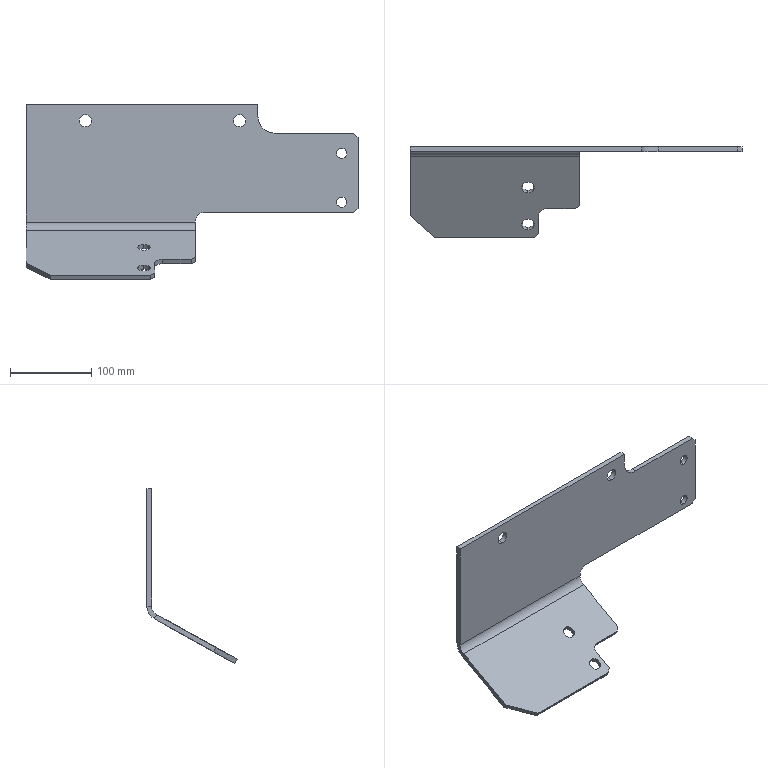Part | SolidWorks | features ICE 2, Chamfer 1, FlatPattern 1, SMBaseFlange 1, SheetMetal 1 | 1 solid | 40 faces | box 408 x 110.914 x 215 mm | volume 454933 mm3 | plane 23 | cylinder 17 | commonest cylinder face diameters 15 x8 12.5 x4 20 x2 24 x1 36 x1 40 x1
STEP:
#1=CARTESIAN_POINT('',(145.,-56.279,-179.402));
#2=VERTEX_POINT('',#1);
#3=CARTESIAN_POINT('',(145.,-43.167,-172.118));
#4=VERTEX_POINT('',#3);
#5=CARTESIAN_POINT('',(145.,-49.723,-175.76));
#6=DIRECTION('',(0.,0.4856,-0.8742));
#7=DIRECTION('',(0.,0.8742,0.4856));
#8=AXIS2_PLACEMENT_3D('',#5,#6,#7);
#9=CIRCLE('',#8,7.5);
#10=EDGE_CURVE('',#2,#4,#9,.T.);
#11=ORIENTED_EDGE('',*,*,#10,.F.);
#12=CARTESIAN_POINT('',(145.,-53.365,-184.647));
#13=VERTEX_POINT('',#12);
#14=CARTESIAN_POINT('',(145.,-145.326,-19.118));
#15=DIRECTION('',(0.,0.4856,-0.8742));
#16=VECTOR('',#15,1000.);
#17=LINE('',#14,#16);
#18=EDGE_CURVE('',#2,#13,#17,.T.);
#19=ORIENTED_EDGE('',*,*,#18,.T.);
#20=CARTESIAN_POINT('',(145.,-40.253,-177.363));
#21=VERTEX_POINT('',#20);
#22=CARTESIAN_POINT('',(145.,-46.809,-181.005));
#23=DIRECTION('',(0.,0.4856,-0.8742));
#24=DIRECTION('',(0.,0.8742,0.4856));
#25=AXIS2_PLACEMENT_3D('',#22,#23,#24);
#26=CIRCLE('',#25,7.5);
#27=EDGE_CURVE('',#13,#21,#26,.T.);
#28=ORIENTED_EDGE('',*,*,#27,.T.);
#29=CARTESIAN_POINT('',(145.,-132.214,-11.833));
#30=DIRECTION('',(0.,0.4856,-0.8742));
#31=VECTOR('',#30,1000.);
#32=LINE('',#29,#31);
#33=EDGE_CURVE('',#4,#21,#32,.T.);
#34=ORIENTED_EDGE('',*,*,#33,.F.);
#35=EDGE_LOOP('',(#11,#19,#28,#34));
#36=FACE_OUTER_BOUND('',#35,.T.);
#37=CARTESIAN_POINT('',(145.,-138.77,-15.476));
#38=DIRECTION('',(0.,0.4856,-0.8742));
#39=DIRECTION('',(0.,0.8742,0.4856));
#40=AXIS2_PLACEMENT_3D('',#37,#38,#39);
#41=CYLINDRICAL_SURFACE('',#40,7.5);
#42=ADVANCED_FACE('',(#36),#41,.F.);
#43=CARTESIAN_POINT('',(145.,-101.735,-204.656));
#44=VERTEX_POINT('',#43);
#45=CARTESIAN_POINT('',(145.,-88.623,-197.371));
#46=VERTEX_POINT('',#45);
#47=CARTESIAN_POINT('',(145.,-95.179,-201.013));
#48=DIRECTION('',(0.,0.4856,-0.8742));
#49=DIRECTION('',(0.,0.8742,0.4856));
#50=AXIS2_PLACEMENT_3D('',#47,#48,#49);
#51=CIRCLE('',#50,7.5);
#52=EDGE_CURVE('',#44,#46,#51,.T.);
#53=ORIENTED_EDGE('',*,*,#52,.F.);
#54=CARTESIAN_POINT('',(145.,-98.821,-209.901));
#55=VERTEX_POINT('',#54);
#56=CARTESIAN_POINT('',(145.,-190.782,-44.371));
#57=DIRECTION('',(0.,0.4856,-0.8742));
#58=VECTOR('',#57,1000.);
#59=LINE('',#56,#58);
#60=EDGE_CURVE('',#44,#55,#59,.T.);
#61=ORIENTED_EDGE('',*,*,#60,.T.);
#62=CARTESIAN_POINT('',(145.,-85.709,-202.616));
#63=VERTEX_POINT('',#62);
#64=CARTESIAN_POINT('',(145.,-92.265,-206.258));
#65=DIRECTION('',(0.,0.4856,-0.8742));
#66=DIRECTION('',(0.,0.8742,0.4856));
#67=AXIS2_PLACEMENT_3D('',#64,#65,#66);
#68=CIRCLE('',#67,7.5);
#69=EDGE_CURVE('',#55,#63,#68,.T.);
#70=ORIENTED_EDGE('',*,*,#69,.T.);
#71=CARTESIAN_POINT('',(145.,-177.67,-37.087));
#72=DIRECTION('',(0.,0.4856,-0.8742));
#73=VECTOR('',#72,1000.);
#74=LINE('',#71,#73);
#75=EDGE_CURVE('',#46,#63,#74,.T.);
#76=ORIENTED_EDGE('',*,*,#75,.F.);
#77=EDGE_LOOP('',(#53,#61,#70,#76));
#78=FACE_OUTER_BOUND('',#77,.T.);
#79=CARTESIAN_POINT('',(145.,-184.226,-40.729));
#80=DIRECTION('',(0.,0.4856,-0.8742));
#81=DIRECTION('',(0.,0.8742,0.4856));
#82=AXIS2_PLACEMENT_3D('',#79,#80,#81);
#83=CYLINDRICAL_SURFACE('',#82,7.5);
#84=ADVANCED_FACE('',(#78),#83,.F.);
#85=CARTESIAN_POINT('',(73.,-6.,-27.5));
#86=VERTEX_POINT('',#85);
#87=CARTESIAN_POINT('',(73.,-6.,-12.5));
#88=VERTEX_POINT('',#87);
#89=CARTESIAN_POINT('',(73.,-6.,-20.));
#90=DIRECTION('',(0.,1.,0.));
#91=DIRECTION('',(0.,0.,1.));
#92=AXIS2_PLACEMENT_3D('',#89,#90,#91);
#93=CIRCLE('',#92,7.5);
#94=EDGE_CURVE('',#86,#88,#93,.T.);
#95=ORIENTED_EDGE('',*,*,#94,.F.);
#96=CARTESIAN_POINT('',(73.,0.,-27.5));
#97=VERTEX_POINT('',#96);
#98=CARTESIAN_POINT('',(73.,-110.914,-27.5));
#99=DIRECTION('',(0.,1.,0.));
#100=VECTOR('',#99,1000.);
#101=LINE('',#98,#100);
#102=EDGE_CURVE('',#86,#97,#101,.T.);
#103=ORIENTED_EDGE('',*,*,#102,.T.);
#104=CARTESIAN_POINT('',(73.,0.,-12.5));
#105=VERTEX_POINT('',#104);
#106=CARTESIAN_POINT('',(73.,0.,-20.));
#107=DIRECTION('',(0.,1.,0.));
#108=DIRECTION('',(0.,0.,1.));
#109=AXIS2_PLACEMENT_3D('',#106,#107,#108);
#110=CIRCLE('',#109,7.5);
#111=EDGE_CURVE('',#97,#105,#110,.T.);
#112=ORIENTED_EDGE('',*,*,#111,.T.);
#113=CARTESIAN_POINT('',(73.,-110.914,-12.5));
#114=DIRECTION('',(0.,1.,0.));
#115=VECTOR('',#114,1000.);
#116=LINE('',#113,#115);
#117=EDGE_CURVE('',#88,#105,#116,.T.);
#118=ORIENTED_EDGE('',*,*,#117,.F.);
#119=EDGE_LOOP('',(#95,#103,#112,#118));
#120=FACE_OUTER_BOUND('',#119,.T.);
#121=CARTESIAN_POINT('',(73.,-110.914,-20.));
#122=DIRECTION('',(0.,1.,0.));
#123=DIRECTION('',(0.,0.,1.));
#124=AXIS2_PLACEMENT_3D('',#121,#122,#123);
#125=CYLINDRICAL_SURFACE('',#124,7.5);
#126=ADVANCED_FACE('',(#120),#125,.F.);
#127=CARTESIAN_POINT('',(388.,-6.,-126.25));
#128=VERTEX_POINT('',#127);
#129=CARTESIAN_POINT('',(388.,-6.,-113.75));
#130=VERTEX_POINT('',#129);
#131=CARTESIAN_POINT('',(388.,-6.,-120.));
#132=DIRECTION('',(0.,1.,0.));
#133=DIRECTION('',(0.,0.,1.));
#134=AXIS2_PLACEMENT_3D('',#131,#132,#133);
#135=CIRCLE('',#134,6.25);
#136=EDGE_CURVE('',#128,#130,#135,.T.);
#137=ORIENTED_EDGE('',*,*,#136,.F.);
#138=CARTESIAN_POINT('',(388.,0.,-126.25));
#139=VERTEX_POINT('',#138);
#140=CARTESIAN_POINT('',(388.,-110.914,-126.25));
#141=DIRECTION('',(0.,1.,0.));
#142=VECTOR('',#141,1000.);
#143=LINE('',#140,#142);
#144=EDGE_CURVE('',#128,#139,#143,.T.);
#145=ORIENTED_EDGE('',*,*,#144,.T.);
#146=CARTESIAN_POINT('',(388.,0.,-113.75));
#147=VERTEX_POINT('',#146);
#148=CARTESIAN_POINT('',(388.,0.,-120.));
#149=DIRECTION('',(0.,1.,0.));
#150=DIRECTION('',(0.,0.,1.));
#151=AXIS2_PLACEMENT_3D('',#148,#149,#150);
#152=CIRCLE('',#151,6.25);
#153=EDGE_CURVE('',#139,#147,#152,.T.);
#154=ORIENTED_EDGE('',*,*,#153,.T.);
#155=CARTESIAN_POINT('',(388.,-110.914,-113.75));
#156=DIRECTION('',(0.,1.,0.));
#157=VECTOR('',#156,1000.);
#158=LINE('',#155,#157);
#159=EDGE_CURVE('',#130,#147,#158,.T.);
#160=ORIENTED_EDGE('',*,*,#159,.F.);
#161=EDGE_LOOP('',(#137,#145,#154,#160));
#162=FACE_OUTER_BOUND('',#161,.T.);
#163=CARTESIAN_POINT('',(388.,-110.914,-120.));
#164=DIRECTION('',(0.,1.,0.));
#165=DIRECTION('',(0.,0.,1.));
#166=AXIS2_PLACEMENT_3D('',#163,#164,#165);
#167=CYLINDRICAL_SURFACE('',#166,6.25);
#168=ADVANCED_FACE('',(#162),#167,.F.);
#169=CARTESIAN_POINT('',(388.,-6.,-66.25));
#170=VERTEX_POINT('',#169);
#171=CARTESIAN_POINT('',(388.,-6.,-53.75));
#172=VERTEX_POINT('',#171);
#173=CARTESIAN_POINT('',(388.,-6.,-60.));
#174=DIRECTION('',(0.,1.,0.));
#175=DIRECTION('',(0.,0.,1.));
#176=AXIS2_PLACEMENT_3D('',#173,#174,#175);
#177=CIRCLE('',#176,6.25);
#178=EDGE_CURVE('',#170,#172,#177,.T.);
#179=ORIENTED_EDGE('',*,*,#178,.F.);
#180=CARTESIAN_POINT('',(388.,0.,-66.25));
#181=VERTEX_POINT('',#180);
#182=CARTESIAN_POINT('',(388.,-110.914,-66.25));
#183=DIRECTION('',(0.,1.,0.));
#184=VECTOR('',#183,1000.);
#185=LINE('',#182,#184);
#186=EDGE_CURVE('',#170,#181,#185,.T.);
#187=ORIENTED_EDGE('',*,*,#186,.T.);
#188=CARTESIAN_POINT('',(388.,0.,-53.75));
#189=VERTEX_POINT('',#188);
#190=CARTESIAN_POINT('',(388.,0.,-60.));
#191=DIRECTION('',(0.,1.,0.));
#192=DIRECTION('',(0.,0.,1.));
#193=AXIS2_PLACEMENT_3D('',#190,#191,#192);
#194=CIRCLE('',#193,6.25);
#195=EDGE_CURVE('',#181,#189,#194,.T.);
#196=ORIENTED_EDGE('',*,*,#195,.T.);
#197=CARTESIAN_POINT('',(388.,-110.914,-53.75));
#198=DIRECTION('',(0.,1.,0.));
#199=VECTOR('',#198,1000.);
#200=LINE('',#197,#199);
#201=EDGE_CURVE('',#172,#189,#200,.T.);
#202=ORIENTED_EDGE('',*,*,#201,.F.);
#203=EDGE_LOOP('',(#179,#187,#196,#202));
#204=FACE_OUTER_BOUND('',#203,.T.);
#205=CARTESIAN_POINT('',(388.,-110.914,-60.));
#206=DIRECTION('',(0.,1.,0.));
#207=DIRECTION('',(0.,0.,1.));
#208=AXIS2_PLACEMENT_3D('',#205,#206,#207);
#209=CYLINDRICAL_SURFACE('',#208,6.25);
#210=ADVANCED_FACE('',(#204),#209,.F.);
#211=CARTESIAN_POINT('',(262.5,-6.,-27.5));
#212=VERTEX_POINT('',#211);
#213=CARTESIAN_POINT('',(262.5,-6.,-12.5));
#214=VERTEX_POINT('',#213);
#215=CARTESIAN_POINT('',(262.5,-6.,-20.));
#216=DIRECTION('',(0.,1.,0.));
#217=DIRECTION('',(0.,0.,1.));
#218=AXIS2_PLACEMENT_3D('',#215,#216,#217);
#219=CIRCLE('',#218,7.5);
#220=EDGE_CURVE('',#212,#214,#219,.T.);
#221=ORIENTED_EDGE('',*,*,#220,.F.);
#222=CARTESIAN_POINT('',(262.5,0.,-27.5));
#223=VERTEX_POINT('',#222);
#224=CARTESIAN_POINT('',(262.5,-110.914,-27.5));
#225=DIRECTION('',(0.,1.,0.));
#226=VECTOR('',#225,1000.);
#227=LINE('',#224,#226);
#228=EDGE_CURVE('',#212,#223,#227,.T.);
#229=ORIENTED_EDGE('',*,*,#228,.T.);
#230=CARTESIAN_POINT('',(262.5,0.,-12.5));
#231=VERTEX_POINT('',#230);
#232=CARTESIAN_POINT('',(262.5,0.,-20.));
#233=DIRECTION('',(0.,1.,0.));
#234=DIRECTION('',(0.,0.,1.));
#235=AXIS2_PLACEMENT_3D('',#232,#233,#234);
#236=CIRCLE('',#235,7.5);
#237=EDGE_CURVE('',#223,#231,#236,.T.);
#238=ORIENTED_EDGE('',*,*,#237,.T.);
#239=CARTESIAN_POINT('',(262.5,-110.914,-12.5));
#240=DIRECTION('',(0.,1.,0.));
#241=VECTOR('',#240,1000.);
#242=LINE('',#239,#241);
#243=EDGE_CURVE('',#214,#231,#242,.T.);
#244=ORIENTED_EDGE('',*,*,#243,.F.);
#245=EDGE_LOOP('',(#221,#229,#238,#244));
#246=FACE_OUTER_BOUND('',#245,.T.);
#247=CARTESIAN_POINT('',(262.5,-110.914,-20.));
#248=DIRECTION('',(0.,1.,0.));
#249=DIRECTION('',(0.,0.,1.));
#250=AXIS2_PLACEMENT_3D('',#247,#248,#249);
#251=CYLINDRICAL_SURFACE('',#250,7.5);
#252=ADVANCED_FACE('',(#246),#251,.F.);
#253=CARTESIAN_POINT('',(208.,-6.,-144.409));
#254=VERTEX_POINT('',#253);
#255=CARTESIAN_POINT('',(208.,-6.,-143.));
#256=VERTEX_POINT('',#255);
#257=CARTESIAN_POINT('',(208.,-6.,0.));
#258=DIRECTION('',(0.,0.,1.));
#259=VECTOR('',#258,1000.);
#260=LINE('',#257,#259);
#261=EDGE_CURVE('',#254,#256,#260,.T.);
#262=ORIENTED_EDGE('',*,*,#261,.F.);
#263=CARTESIAN_POINT('',(208.,0.,-144.409));
#264=VERTEX_POINT('',#263);
#265=CARTESIAN_POINT('',(208.,-6.,-144.409));
#266=DIRECTION('',(0.,1.,0.));
#267=VECTOR('',#266,1000.);
#268=LINE('',#265,#267);
#269=EDGE_CURVE('',#254,#264,#268,.T.);
#270=ORIENTED_EDGE('',*,*,#269,.T.);
#271=CARTESIAN_POINT('',(208.,0.,-143.));
#272=VERTEX_POINT('',#271);
#273=CARTESIAN_POINT('',(208.,0.,-143.));
#274=DIRECTION('',(0.,0.,1.));
#275=VECTOR('',#274,1000.);
#276=LINE('',#273,#275);
#277=EDGE_CURVE('',#264,#272,#276,.T.);
#278=ORIENTED_EDGE('',*,*,#277,.T.);
#279=CARTESIAN_POINT('',(208.,-110.914,-143.));
#280=DIRECTION('',(0.,1.,0.));
#281=VECTOR('',#280,1000.);
#282=LINE('',#279,#281);
#283=EDGE_CURVE('',#256,#272,#282,.T.);
#284=ORIENTED_EDGE('',*,*,#283,.F.);
#285=EDGE_LOOP('',(#262,#270,#278,#284));
#286=FACE_OUTER_BOUND('',#285,.T.);
#287=CARTESIAN_POINT('',(208.,-110.914,-143.));
#288=DIRECTION('',(-1.,0.,0.));
#289=DIRECTION('',(0.,0.,1.));
#290=AXIS2_PLACEMENT_3D('',#287,#288,#289);
#291=PLANE('',#290);
#292=ADVANCED_FACE('',(#286),#291,.F.);
#293=CARTESIAN_POINT('',(208.,-71.577,-187.901));
#294=VERTEX_POINT('',#293);
#295=CARTESIAN_POINT('',(208.,-12.172,-154.899));
#296=VERTEX_POINT('',#295);
#297=CARTESIAN_POINT('',(208.,-2.914,-149.755));
#298=DIRECTION('',(0.,0.8742,0.4856));
#299=VECTOR('',#298,1000.);
#300=LINE('',#297,#299);
#301=EDGE_CURVE('',#294,#296,#300,.T.);
#302=ORIENTED_EDGE('',*,*,#301,.F.);
#303=CARTESIAN_POINT('',(208.,-68.663,-193.146));
#304=VERTEX_POINT('',#303);
#305=CARTESIAN_POINT('',(208.,-99.916,-136.89));
#306=DIRECTION('',(0.,0.4856,-0.8742));
#307=VECTOR('',#306,1000.);
#308=LINE('',#305,#307);
#309=EDGE_CURVE('',#294,#304,#308,.T.);
#310=ORIENTED_EDGE('',*,*,#309,.T.);
#311=CARTESIAN_POINT('',(208.,-9.258,-160.144));
#312=VERTEX_POINT('',#311);
#313=CARTESIAN_POINT('',(208.,0.,-155.));
#314=DIRECTION('',(0.,0.8742,0.4856));
#315=VECTOR('',#314,1000.);
#316=LINE('',#313,#315);
#317=EDGE_CURVE('',#304,#312,#316,.T.);
#318=ORIENTED_EDGE('',*,*,#317,.T.);
#319=CARTESIAN_POINT('',(208.,-9.258,-160.144));
#320=DIRECTION('',(0.,-0.4856,0.8742));
#321=VECTOR('',#320,1000.);
#322=LINE('',#319,#321);
#323=EDGE_CURVE('',#312,#296,#322,.T.);
#324=ORIENTED_EDGE('',*,*,#323,.T.);
#325=EDGE_LOOP('',(#302,#310,#318,#324));
#326=FACE_OUTER_BOUND('',#325,.T.);
#327=CARTESIAN_POINT('',(208.,-110.914,-143.));
#328=DIRECTION('',(-1.,0.,0.));
#329=DIRECTION('',(0.,0.,1.));
#330=AXIS2_PLACEMENT_3D('',#327,#328,#329);
#331=PLANE('',#330);
#332=ADVANCED_FACE('',(#326),#331,.F.);
#333=CARTESIAN_POINT('',(0.,0.,-144.409));
#334=VERTEX_POINT('',#333);
#335=CARTESIAN_POINT('',(0.,-6.,-144.409));
#336=VERTEX_POINT('',#335);
#337=CARTESIAN_POINT('',(0.,0.,-144.409));
#338=DIRECTION('',(0.,-1.,0.));
#339=VECTOR('',#338,1000.);
#340=LINE('',#337,#339);
#341=EDGE_CURVE('',#334,#336,#340,.T.);
#342=ORIENTED_EDGE('',*,*,#341,.F.);
#343=CARTESIAN_POINT('',(0.,-9.258,-160.144));
#344=VERTEX_POINT('',#343);
#345=CARTESIAN_POINT('',(0.,-18.,-144.409));
#346=DIRECTION('',(-1.,0.,0.));
#347=DIRECTION('',(0.,0.,-1.));
#348=AXIS2_PLACEMENT_3D('',#345,#346,#347);
#349=CIRCLE('',#348,18.);
#350=EDGE_CURVE('',#334,#344,#349,.T.);
#351=ORIENTED_EDGE('',*,*,#350,.T.);
#352=CARTESIAN_POINT('',(0.,-12.172,-154.899));
#353=VERTEX_POINT('',#352);
#354=CARTESIAN_POINT('',(0.,-12.172,-154.899));
#355=DIRECTION('',(0.,0.4856,-0.8742));
#356=VECTOR('',#355,1000.);
#357=LINE('',#354,#356);
#358=EDGE_CURVE('',#353,#344,#357,.T.);
#359=ORIENTED_EDGE('',*,*,#358,.F.);
#360=CARTESIAN_POINT('',(0.,-18.,-144.409));
#361=DIRECTION('',(-1.,0.,0.));
#362=DIRECTION('',(0.,0.,-1.));
#363=AXIS2_PLACEMENT_3D('',#360,#361,#362);
#364=CIRCLE('',#363,12.);
#365=EDGE_CURVE('',#336,#353,#364,.T.);
#366=ORIENTED_EDGE('',*,*,#365,.F.);
#367=EDGE_LOOP('',(#342,#351,#359,#366));
#368=FACE_OUTER_BOUND('',#367,.T.);
#369=CARTESIAN_POINT('',(0.,0.,-144.409));
#370=DIRECTION('',(-1.,0.,0.));
#371=DIRECTION('',(0.,0.,1.));
#372=AXIS2_PLACEMENT_3D('',#369,#370,#371);
#373=PLANE('',#372);
#374=ADVANCED_FACE('',(#368),#373,.T.);
#375=CARTESIAN_POINT('',(0.,0.,0.));
#376=VERTEX_POINT('',#375);
#377=CARTESIAN_POINT('',(0.,0.,0.));
#378=DIRECTION('',(0.,0.,-1.));
#379=VECTOR('',#378,1000.);
#380=LINE('',#377,#379);
#381=EDGE_CURVE('',#376,#334,#380,.T.);
#382=ORIENTED_EDGE('',*,*,#381,.T.);
#383=ORIENTED_EDGE('',*,*,#341,.T.);
#384=CARTESIAN_POINT('',(0.,-6.,0.));
#385=VERTEX_POINT('',#384);
#386=CARTESIAN_POINT('',(0.,-6.,0.));
#387=DIRECTION('',(0.,0.,-1.));
#388=VECTOR('',#387,1000.);
#389=LINE('',#386,#388);
#390=EDGE_CURVE('',#385,#336,#389,.T.);
#391=ORIENTED_EDGE('',*,*,#390,.F.);
#392=CARTESIAN_POINT('',(0.,-6.,0.));
#393=DIRECTION('',(0.,1.,0.));
#394=VECTOR('',#393,1000.);
#395=LINE('',#392,#394);
#396=EDGE_CURVE('',#385,#376,#395,.T.);
#397=ORIENTED_EDGE('',*,*,#396,.T.);
#398=EDGE_LOOP('',(#382,#383,#391,#397));
#399=FACE_OUTER_BOUND('',#398,.T.);
#400=CARTESIAN_POINT('',(0.,-12.172,-154.899));
#401=DIRECTION('',(-1.,0.,0.));
#402=DIRECTION('',(0.,0.,1.));
#403=AXIS2_PLACEMENT_3D('',#400,#401,#402);
#404=PLANE('',#403);
#405=ADVANCED_FACE('',(#399),#404,.T.);
#406=CARTESIAN_POINT('',(145.,-49.723,-175.76));
#407=DIRECTION('',(0.,0.4856,-0.8742));
#408=DIRECTION('',(0.,0.8742,0.4856));
#409=AXIS2_PLACEMENT_3D('',#406,#407,#408);
#410=CIRCLE('',#409,7.5);
#411=EDGE_CURVE('',#4,#2,#410,.T.);
#412=ORIENTED_EDGE('',*,*,#411,.T.);
#413=ORIENTED_EDGE('',*,*,#10,.T.);
#414=EDGE_LOOP('',(#412,#413));
#415=FACE_BOUND('',#414,.T.);
#416=CARTESIAN_POINT('',(145.,-95.179,-201.013));
#417=DIRECTION('',(0.,0.4856,-0.8742));
#418=DIRECTION('',(0.,0.8742,0.4856));
#419=AXIS2_PLACEMENT_3D('',#416,#417,#418);
#420=CIRCLE('',#419,7.5);
#421=EDGE_CURVE('',#46,#44,#420,.T.);
#422=ORIENTED_EDGE('',*,*,#421,.T.);
#423=ORIENTED_EDGE('',*,*,#52,.T.);
#424=EDGE_LOOP('',(#422,#423));
#425=FACE_BOUND('',#424,.T.);
#426=CARTESIAN_POINT('',(153.,-110.914,-209.755));
#427=VERTEX_POINT('',#426);
#428=CARTESIAN_POINT('',(30.,-110.914,-209.755));
#429=VERTEX_POINT('',#428);
#430=CARTESIAN_POINT('',(408.,-110.914,-209.755));
#431=DIRECTION('',(-1.,0.,0.));
#432=VECTOR('',#431,1000.);
#433=LINE('',#430,#432);
#434=EDGE_CURVE('',#427,#429,#433,.T.);
#435=ORIENTED_EDGE('',*,*,#434,.F.);
#436=CARTESIAN_POINT('',(158.,-106.543,-207.327));
#437=VERTEX_POINT('',#436);
#438=CARTESIAN_POINT('',(158.,-106.543,-207.327));
#439=DIRECTION('',(0.7071,0.6181,0.3434));
#440=VECTOR('',#439,1000.);
#441=LINE('',#438,#440);
#442=EDGE_CURVE('',#427,#437,#441,.T.);
#443=ORIENTED_EDGE('',*,*,#442,.T.);
#444=CARTESIAN_POINT('',(158.,-84.689,-195.186));
#445=VERTEX_POINT('',#444);
#446=CARTESIAN_POINT('',(158.,-2.914,-149.755));
#447=DIRECTION('',(0.,0.8742,0.4856));
#448=VECTOR('',#447,1000.);
#449=LINE('',#446,#448);
#450=EDGE_CURVE('',#437,#445,#449,.T.);
#451=ORIENTED_EDGE('',*,*,#450,.T.);
#452=CARTESIAN_POINT('',(168.,-75.948,-190.329));
#453=VERTEX_POINT('',#452);
#454=CARTESIAN_POINT('',(168.,-84.689,-195.186));
#455=DIRECTION('',(0.,0.4856,-0.8742));
#456=DIRECTION('',(0.,0.8742,0.4856));
#457=AXIS2_PLACEMENT_3D('',#454,#455,#456);
#458=CIRCLE('',#457,10.);
#459=EDGE_CURVE('',#445,#453,#458,.T.);
#460=ORIENTED_EDGE('',*,*,#459,.T.);
#461=CARTESIAN_POINT('',(203.,-75.948,-190.329));
#462=VERTEX_POINT('',#461);
#463=CARTESIAN_POINT('',(408.,-75.948,-190.329));
#464=DIRECTION('',(1.,0.,0.));
#465=VECTOR('',#464,1000.);
#466=LINE('',#463,#465);
#467=EDGE_CURVE('',#453,#462,#466,.T.);
#468=ORIENTED_EDGE('',*,*,#467,.T.);
#469=CARTESIAN_POINT('',(208.,-71.577,-187.901));
#470=DIRECTION('',(0.7071,0.6181,0.3434));
#471=VECTOR('',#470,1000.);
#472=LINE('',#469,#471);
#473=EDGE_CURVE('',#462,#294,#472,.T.);
#474=ORIENTED_EDGE('',*,*,#473,.T.);
#475=ORIENTED_EDGE('',*,*,#301,.T.);
#476=CARTESIAN_POINT('',(408.,-12.172,-154.899));
#477=DIRECTION('',(-1.,0.,0.));
#478=VECTOR('',#477,1000.);
#479=LINE('',#476,#478);
#480=EDGE_CURVE('',#296,#353,#479,.T.);
#481=ORIENTED_EDGE('',*,*,#480,.T.);
#482=CARTESIAN_POINT('',(0.,-84.689,-195.186));
#483=VERTEX_POINT('',#482);
#484=CARTESIAN_POINT('',(0.,-2.914,-149.755));
#485=DIRECTION('',(0.,-0.8742,-0.4856));
#486=VECTOR('',#485,1000.);
#487=LINE('',#484,#486);
#488=EDGE_CURVE('',#353,#483,#487,.T.);
#489=ORIENTED_EDGE('',*,*,#488,.T.);
#490=CARTESIAN_POINT('',(157.226,-222.13,-271.542));
#491=DIRECTION('',(0.7071,-0.6181,-0.3434));
#492=VECTOR('',#491,1000.);
#493=LINE('',#490,#492);
#494=EDGE_CURVE('',#483,#429,#493,.T.);
#495=ORIENTED_EDGE('',*,*,#494,.T.);
#496=EDGE_LOOP('',(#435,#443,#451,#460,#468,#474,#475,#481,#489,#495));
#497=FACE_OUTER_BOUND('',#496,.T.);
#498=CARTESIAN_POINT('',(408.,-2.914,-149.755));
#499=DIRECTION('',(0.,0.4856,-0.8742));
#500=DIRECTION('',(0.,0.8742,0.4856));
#501=AXIS2_PLACEMENT_3D('',#498,#499,#500);
#502=PLANE('',#501);
#503=ADVANCED_FACE('',(#415,#425,#497),#502,.F.);
#504=CARTESIAN_POINT('',(153.,-108.,-215.));
#505=VERTEX_POINT('',#504);
#506=CARTESIAN_POINT('',(30.,-108.,-215.));
#507=VERTEX_POINT('',#506);
#508=CARTESIAN_POINT('',(408.,-108.,-215.));
#509=DIRECTION('',(-1.,0.,0.));
#510=VECTOR('',#509,1000.);
#511=LINE('',#508,#510);
#512=EDGE_CURVE('',#505,#507,#511,.T.);
#513=ORIENTED_EDGE('',*,*,#512,.F.);
#514=CARTESIAN_POINT('',(153.,-110.914,-209.755));
#515=DIRECTION('',(0.,-0.4856,0.8742));
#516=VECTOR('',#515,1000.);
#517=LINE('',#514,#516);
#518=EDGE_CURVE('',#505,#427,#517,.T.);
#519=ORIENTED_EDGE('',*,*,#518,.T.);
#520=ORIENTED_EDGE('',*,*,#434,.T.);
#521=CARTESIAN_POINT('',(30.,-199.961,-49.471));
#522=DIRECTION('',(0.,0.4856,-0.8742));
#523=VECTOR('',#522,1000.);
#524=LINE('',#521,#523);
#525=EDGE_CURVE('',#429,#507,#524,.T.);
#526=ORIENTED_EDGE('',*,*,#525,.T.);
#527=EDGE_LOOP('',(#513,#519,#520,#526));
#528=FACE_OUTER_BOUND('',#527,.T.);
#529=CARTESIAN_POINT('',(408.,-108.,-215.));
#530=DIRECTION('',(0.,-0.8742,-0.4856));
#531=DIRECTION('',(0.,0.4856,-0.8742));
#532=AXIS2_PLACEMENT_3D('',#529,#530,#531);
#533=PLANE('',#532);
#534=ADVANCED_FACE('',(#528),#533,.T.);
#535=CARTESIAN_POINT('',(158.,-103.629,-212.572));
#536=VERTEX_POINT('',#535);
#537=CARTESIAN_POINT('',(158.,-81.775,-200.431));
#538=VERTEX_POINT('',#537);
#539=CARTESIAN_POINT('',(158.,-81.775,-200.431));
#540=DIRECTION('',(0.,0.8742,0.4856));
#541=VECTOR('',#540,1000.);
#542=LINE('',#539,#541);
#543=EDGE_CURVE('',#536,#538,#542,.T.);
#544=ORIENTED_EDGE('',*,*,#543,.F.);
#545=CARTESIAN_POINT('',(342.274,57.455,-123.081));
#546=DIRECTION('',(-0.7071,-0.6181,-0.3434));
#547=VECTOR('',#546,1000.);
#548=LINE('',#545,#547);
#549=EDGE_CURVE('',#536,#505,#548,.T.);
#550=ORIENTED_EDGE('',*,*,#549,.T.);
#551=ORIENTED_EDGE('',*,*,#512,.T.);
#552=CARTESIAN_POINT('',(0.,-81.775,-200.431));
#553=VERTEX_POINT('',#552);
#554=CARTESIAN_POINT('',(30.,-108.,-215.));
#555=DIRECTION('',(0.7071,-0.6181,-0.3434));
#556=VECTOR('',#555,1000.);
#557=LINE('',#554,#556);
#558=EDGE_CURVE('',#553,#507,#557,.T.);
#559=ORIENTED_EDGE('',*,*,#558,.F.);
#560=CARTESIAN_POINT('',(0.,0.,-155.));
#561=DIRECTION('',(0.,-0.8742,-0.4856));
#562=VECTOR('',#561,1000.);
#563=LINE('',#560,#562);
#564=EDGE_CURVE('',#344,#553,#563,.T.);
#565=ORIENTED_EDGE('',*,*,#564,.F.);
#566=CARTESIAN_POINT('',(408.,-9.258,-160.144));
#567=DIRECTION('',(-1.,0.,0.));
#568=VECTOR('',#567,1000.);
#569=LINE('',#566,#568);
#570=EDGE_CURVE('',#312,#344,#569,.T.);
#571=ORIENTED_EDGE('',*,*,#570,.F.);
#572=ORIENTED_EDGE('',*,*,#317,.F.);
#573=CARTESIAN_POINT('',(203.,-73.034,-195.574));
#574=VERTEX_POINT('',#573);
#575=CARTESIAN_POINT('',(347.274,53.084,-125.509));
#576=DIRECTION('',(-0.7071,-0.6181,-0.3434));
#577=VECTOR('',#576,1000.);
#578=LINE('',#575,#577);
#579=EDGE_CURVE('',#304,#574,#578,.T.);
#580=ORIENTED_EDGE('',*,*,#579,.T.);
#581=CARTESIAN_POINT('',(168.,-73.034,-195.574));
#582=VERTEX_POINT('',#581);
#583=CARTESIAN_POINT('',(208.,-73.034,-195.574));
#584=DIRECTION('',(1.,0.,0.));
#585=VECTOR('',#584,1000.);
#586=LINE('',#583,#585);
#587=EDGE_CURVE('',#582,#574,#586,.T.);
#588=ORIENTED_EDGE('',*,*,#587,.F.);
#589=CARTESIAN_POINT('',(168.,-81.775,-200.431));
#590=DIRECTION('',(0.,0.4856,-0.8742));
#591=DIRECTION('',(0.,-0.8742,-0.4856));
#592=AXIS2_PLACEMENT_3D('',#589,#590,#591);
#593=CIRCLE('',#592,10.);
#594=EDGE_CURVE('',#538,#582,#593,.T.);
#595=ORIENTED_EDGE('',*,*,#594,.F.);
#596=EDGE_LOOP('',(#544,#550,#551,#559,#565,#571,#572,#580,#588,#595));
#597=FACE_OUTER_BOUND('',#596,.T.);
#598=CARTESIAN_POINT('',(145.,-46.809,-181.005));
#599=DIRECTION('',(0.,0.4856,-0.8742));
#600=DIRECTION('',(0.,0.8742,0.4856));
#601=AXIS2_PLACEMENT_3D('',#598,#599,#600);
#602=CIRCLE('',#601,7.5);
#603=EDGE_CURVE('',#21,#13,#602,.T.);
#604=ORIENTED_EDGE('',*,*,#603,.F.);
#605=ORIENTED_EDGE('',*,*,#27,.F.);
#606=EDGE_LOOP('',(#604,#605));
#607=FACE_BOUND('',#606,.T.);
#608=CARTESIAN_POINT('',(145.,-92.265,-206.258));
#609=DIRECTION('',(0.,0.4856,-0.8742));
#610=DIRECTION('',(0.,0.8742,0.4856));
#611=AXIS2_PLACEMENT_3D('',#608,#609,#610);
#612=CIRCLE('',#611,7.5);
#613=EDGE_CURVE('',#63,#55,#612,.T.);
#614=ORIENTED_EDGE('',*,*,#613,.F.);
#615=ORIENTED_EDGE('',*,*,#69,.F.);
#616=EDGE_LOOP('',(#614,#615));
#617=FACE_BOUND('',#616,.T.);
#618=CARTESIAN_POINT('',(408.,0.,-155.));
#619=DIRECTION('',(0.,0.4856,-0.8742));
#620=DIRECTION('',(0.,0.8742,0.4856));
#621=AXIS2_PLACEMENT_3D('',#618,#619,#620);
#622=PLANE('',#621);
#623=ADVANCED_FACE('',(#597,#607,#617),#622,.T.);
#624=CARTESIAN_POINT('',(208.,-18.,-144.409));
#625=DIRECTION('',(1.,0.,0.));
#626=DIRECTION('',(0.,0.,1.));
#627=AXIS2_PLACEMENT_3D('',#624,#625,#626);
#628=CIRCLE('',#627,18.);
#629=EDGE_CURVE('',#312,#264,#628,.T.);
#630=ORIENTED_EDGE('',*,*,#629,.F.);
#631=ORIENTED_EDGE('',*,*,#570,.T.);
#632=ORIENTED_EDGE('',*,*,#350,.F.);
#633=CARTESIAN_POINT('',(408.,0.,-144.409));
#634=DIRECTION('',(-1.,0.,0.));
#635=VECTOR('',#634,1000.);
#636=LINE('',#633,#635);
#637=EDGE_CURVE('',#264,#334,#636,.T.);
#638=ORIENTED_EDGE('',*,*,#637,.F.);
#639=EDGE_LOOP('',(#630,#631,#632,#638));
#640=FACE_OUTER_BOUND('',#639,.T.);
#641=CARTESIAN_POINT('',(408.,-18.,-144.409));
#642=DIRECTION('',(-1.,0.,0.));
#643=DIRECTION('',(0.,0.,1.));
#644=AXIS2_PLACEMENT_3D('',#641,#642,#643);
#645=CYLINDRICAL_SURFACE('',#644,18.);
#646=ADVANCED_FACE('',(#640),#645,.T.);
#647=CARTESIAN_POINT('',(73.,0.,-20.));
#648=DIRECTION('',(0.,1.,0.));
#649=DIRECTION('',(0.,0.,1.));
#650=AXIS2_PLACEMENT_3D('',#647,#648,#649);
#651=CIRCLE('',#650,7.5);
#652=EDGE_CURVE('',#105,#97,#651,.T.);
#653=ORIENTED_EDGE('',*,*,#652,.F.);
#654=ORIENTED_EDGE('',*,*,#111,.F.);
#655=EDGE_LOOP('',(#653,#654));
#656=FACE_BOUND('',#655,.T.);
#657=CARTESIAN_POINT('',(388.,0.,-120.));
#658=DIRECTION('',(0.,1.,0.));
#659=DIRECTION('',(0.,0.,1.));
#660=AXIS2_PLACEMENT_3D('',#657,#658,#659);
#661=CIRCLE('',#660,6.25);
#662=EDGE_CURVE('',#147,#139,#661,.T.);
#663=ORIENTED_EDGE('',*,*,#662,.F.);
#664=ORIENTED_EDGE('',*,*,#153,.F.);
#665=EDGE_LOOP('',(#663,#664));
#666=FACE_BOUND('',#665,.T.);
#667=CARTESIAN_POINT('',(388.,0.,-60.));
#668=DIRECTION('',(0.,1.,0.));
#669=DIRECTION('',(0.,0.,1.));
#670=AXIS2_PLACEMENT_3D('',#667,#668,#669);
#671=CIRCLE('',#670,6.25);
#672=EDGE_CURVE('',#189,#181,#671,.T.);
#673=ORIENTED_EDGE('',*,*,#672,.F.);
#674=ORIENTED_EDGE('',*,*,#195,.F.);
#675=EDGE_LOOP('',(#673,#674));
#676=FACE_BOUND('',#675,.T.);
#677=CARTESIAN_POINT('',(403.,0.,-35.));
#678=VERTEX_POINT('',#677);
#679=CARTESIAN_POINT('',(305.,0.,-35.));
#680=VERTEX_POINT('',#679);
#681=CARTESIAN_POINT('',(305.,0.,-35.));
#682=DIRECTION('',(-1.,0.,0.));
#683=VECTOR('',#682,1000.);
#684=LINE('',#681,#683);
#685=EDGE_CURVE('',#678,#680,#684,.T.);
#686=ORIENTED_EDGE('',*,*,#685,.F.);
#687=CARTESIAN_POINT('',(408.,0.,-40.));
#688=VERTEX_POINT('',#687);
#689=CARTESIAN_POINT('',(388.,0.,-20.));
#690=DIRECTION('',(0.7071,0.,-0.7071));
#691=VECTOR('',#690,1000.);
#692=LINE('',#689,#691);
#693=EDGE_CURVE('',#678,#688,#692,.T.);
#694=ORIENTED_EDGE('',*,*,#693,.T.);
#695=CARTESIAN_POINT('',(408.,0.,-128.));
#696=VERTEX_POINT('',#695);
#697=CARTESIAN_POINT('',(408.,0.,0.));
#698=DIRECTION('',(0.,0.,-1.));
#699=VECTOR('',#698,1000.);
#700=LINE('',#697,#699);
#701=EDGE_CURVE('',#688,#696,#700,.T.);
#702=ORIENTED_EDGE('',*,*,#701,.T.);
#703=CARTESIAN_POINT('',(403.,0.,-133.));
#704=VERTEX_POINT('',#703);
#705=CARTESIAN_POINT('',(472.,0.,-64.));
#706=DIRECTION('',(-0.7071,0.,-0.7071));
#707=VECTOR('',#706,1000.);
#708=LINE('',#705,#707);
#709=EDGE_CURVE('',#696,#704,#708,.T.);
#710=ORIENTED_EDGE('',*,*,#709,.T.);
#711=CARTESIAN_POINT('',(218.,0.,-133.));
#712=VERTEX_POINT('',#711);
#713=CARTESIAN_POINT('',(408.,0.,-133.));
#714=DIRECTION('',(1.,0.,0.));
#715=VECTOR('',#714,1000.);
#716=LINE('',#713,#715);
#717=EDGE_CURVE('',#712,#704,#716,.T.);
#718=ORIENTED_EDGE('',*,*,#717,.F.);
#719=CARTESIAN_POINT('',(218.,0.,-143.));
#720=DIRECTION('',(0.,1.,0.));
#721=DIRECTION('',(0.,0.,-1.));
#722=AXIS2_PLACEMENT_3D('',#719,#720,#721);
#723=CIRCLE('',#722,10.);
#724=EDGE_CURVE('',#272,#712,#723,.T.);
#725=ORIENTED_EDGE('',*,*,#724,.F.);
#726=ORIENTED_EDGE('',*,*,#277,.F.);
#727=ORIENTED_EDGE('',*,*,#637,.T.);
#728=ORIENTED_EDGE('',*,*,#381,.F.);
#729=CARTESIAN_POINT('',(285.,0.,0.));
#730=VERTEX_POINT('',#729);
#731=CARTESIAN_POINT('',(408.,0.,0.));
#732=DIRECTION('',(-1.,0.,0.));
#733=VECTOR('',#732,1000.);
#734=LINE('',#731,#733);
#735=EDGE_CURVE('',#730,#376,#734,.T.);
#736=ORIENTED_EDGE('',*,*,#735,.F.);
#737=CARTESIAN_POINT('',(285.,0.,-15.));
#738=VERTEX_POINT('',#737);
#739=CARTESIAN_POINT('',(285.,0.,0.));
#740=DIRECTION('',(0.,0.,1.));
#741=VECTOR('',#740,1000.);
#742=LINE('',#739,#741);
#743=EDGE_CURVE('',#738,#730,#742,.T.);
#744=ORIENTED_EDGE('',*,*,#743,.F.);
#745=CARTESIAN_POINT('',(305.,0.,-15.));
#746=DIRECTION('',(0.,1.,0.));
#747=DIRECTION('',(0.,0.,-1.));
#748=AXIS2_PLACEMENT_3D('',#745,#746,#747);
#749=CIRCLE('',#748,20.);
#750=EDGE_CURVE('',#680,#738,#749,.T.);
#751=ORIENTED_EDGE('',*,*,#750,.F.);
#752=EDGE_LOOP('',(#686,#694,#702,#710,#718,#725,#726,#727,#728,#736,#744,#751));
#753=FACE_OUTER_BOUND('',#752,.T.);
#754=CARTESIAN_POINT('',(262.5,0.,-20.));
#755=DIRECTION('',(0.,1.,0.));
#756=DIRECTION('',(0.,0.,1.));
#757=AXIS2_PLACEMENT_3D('',#754,#755,#756);
#758=CIRCLE('',#757,7.5);
#759=EDGE_CURVE('',#231,#223,#758,.T.);
#760=ORIENTED_EDGE('',*,*,#759,.F.);
#761=ORIENTED_EDGE('',*,*,#237,.F.);
#762=EDGE_LOOP('',(#760,#761));
#763=FACE_BOUND('',#762,.T.);
#764=CARTESIAN_POINT('',(408.,0.,0.));
#765=DIRECTION('',(0.,1.,0.));
#766=DIRECTION('',(0.,0.,1.));
#767=AXIS2_PLACEMENT_3D('',#764,#765,#766);
#768=PLANE('',#767);
#769=ADVANCED_FACE('',(#656,#666,#676,#753,#763),#768,.T.);
#770=CARTESIAN_POINT('',(285.,-6.,0.));
#771=VERTEX_POINT('',#770);
#772=CARTESIAN_POINT('',(285.,-110.914,0.));
#773=DIRECTION('',(0.,1.,0.));
#774=VECTOR('',#773,1000.);
#775=LINE('',#772,#774);
#776=EDGE_CURVE('',#771,#730,#775,.T.);
#777=ORIENTED_EDGE('',*,*,#776,.T.);
#778=ORIENTED_EDGE('',*,*,#735,.T.);
#779=ORIENTED_EDGE('',*,*,#396,.F.);
#780=CARTESIAN_POINT('',(408.,-6.,0.));
#781=DIRECTION('',(-1.,0.,0.));
#782=VECTOR('',#781,1000.);
#783=LINE('',#780,#782);
#784=EDGE_CURVE('',#771,#385,#783,.T.);
#785=ORIENTED_EDGE('',*,*,#784,.F.);
#786=EDGE_LOOP('',(#777,#778,#779,#785));
#787=FACE_OUTER_BOUND('',#786,.T.);
#788=CARTESIAN_POINT('',(408.,-6.,0.));
#789=DIRECTION('',(0.,0.,1.));
#790=DIRECTION('',(1.,0.,0.));
#791=AXIS2_PLACEMENT_3D('',#788,#789,#790);
#792=PLANE('',#791);
#793=ADVANCED_FACE('',(#787),#792,.T.);
#794=CARTESIAN_POINT('',(73.,-6.,-20.));
#795=DIRECTION('',(0.,1.,0.));
#796=DIRECTION('',(0.,0.,1.));
#797=AXIS2_PLACEMENT_3D('',#794,#795,#796);
#798=CIRCLE('',#797,7.5);
#799=EDGE_CURVE('',#88,#86,#798,.T.);
#800=ORIENTED_EDGE('',*,*,#799,.T.);
#801=ORIENTED_EDGE('',*,*,#94,.T.);
#802=EDGE_LOOP('',(#800,#801));
#803=FACE_BOUND('',#802,.T.);
#804=CARTESIAN_POINT('',(388.,-6.,-120.));
#805=DIRECTION('',(0.,1.,0.));
#806=DIRECTION('',(0.,0.,1.));
#807=AXIS2_PLACEMENT_3D('',#804,#805,#806);
#808=CIRCLE('',#807,6.25);
#809=EDGE_CURVE('',#130,#128,#808,.T.);
#810=ORIENTED_EDGE('',*,*,#809,.T.);
#811=ORIENTED_EDGE('',*,*,#136,.T.);
#812=EDGE_LOOP('',(#810,#811));
#813=FACE_BOUND('',#812,.T.);
#814=CARTESIAN_POINT('',(388.,-6.,-60.));
#815=DIRECTION('',(0.,1.,0.));
#816=DIRECTION('',(0.,0.,1.));
#817=AXIS2_PLACEMENT_3D('',#814,#815,#816);
#818=CIRCLE('',#817,6.25);
#819=EDGE_CURVE('',#172,#170,#818,.T.);
#820=ORIENTED_EDGE('',*,*,#819,.T.);
#821=ORIENTED_EDGE('',*,*,#178,.T.);
#822=EDGE_LOOP('',(#820,#821));
#823=FACE_BOUND('',#822,.T.);
#824=CARTESIAN_POINT('',(262.5,-6.,-20.));
#825=DIRECTION('',(0.,1.,0.));
#826=DIRECTION('',(0.,0.,1.));
#827=AXIS2_PLACEMENT_3D('',#824,#825,#826);
#828=CIRCLE('',#827,7.5);
#829=EDGE_CURVE('',#214,#212,#828,.T.);
#830=ORIENTED_EDGE('',*,*,#829,.T.);
#831=ORIENTED_EDGE('',*,*,#220,.T.);
#832=EDGE_LOOP('',(#830,#831));
#833=FACE_BOUND('',#832,.T.);
#834=CARTESIAN_POINT('',(408.,-6.,-40.));
#835=VERTEX_POINT('',#834);
#836=CARTESIAN_POINT('',(408.,-6.,-128.));
#837=VERTEX_POINT('',#836);
#838=CARTESIAN_POINT('',(408.,-6.,0.));
#839=DIRECTION('',(0.,0.,-1.));
#840=VECTOR('',#839,1000.);
#841=LINE('',#838,#840);
#842=EDGE_CURVE('',#835,#837,#841,.T.);
#843=ORIENTED_EDGE('',*,*,#842,.F.);
#844=CARTESIAN_POINT('',(403.,-6.,-35.));
#845=VERTEX_POINT('',#844);
#846=CARTESIAN_POINT('',(403.,-6.,-35.));
#847=DIRECTION('',(-0.7071,0.,0.7071));
#848=VECTOR('',#847,1000.);
#849=LINE('',#846,#848);
#850=EDGE_CURVE('',#835,#845,#849,.T.);
#851=ORIENTED_EDGE('',*,*,#850,.T.);
#852=CARTESIAN_POINT('',(305.,-6.,-35.));
#853=VERTEX_POINT('',#852);
#854=CARTESIAN_POINT('',(408.,-6.,-35.));
#855=DIRECTION('',(-1.,0.,0.));
#856=VECTOR('',#855,1000.);
#857=LINE('',#854,#856);
#858=EDGE_CURVE('',#845,#853,#857,.T.);
#859=ORIENTED_EDGE('',*,*,#858,.T.);
#860=CARTESIAN_POINT('',(285.,-6.,-15.));
#861=VERTEX_POINT('',#860);
#862=CARTESIAN_POINT('',(305.,-6.,-15.));
#863=DIRECTION('',(0.,1.,0.));
#864=DIRECTION('',(0.,0.,1.));
#865=AXIS2_PLACEMENT_3D('',#862,#863,#864);
#866=CIRCLE('',#865,20.);
#867=EDGE_CURVE('',#853,#861,#866,.T.);
#868=ORIENTED_EDGE('',*,*,#867,.T.);
#869=CARTESIAN_POINT('',(285.,-6.,0.));
#870=DIRECTION('',(0.,0.,1.));
#871=VECTOR('',#870,1000.);
#872=LINE('',#869,#871);
#873=EDGE_CURVE('',#861,#771,#872,.T.);
#874=ORIENTED_EDGE('',*,*,#873,.T.);
#875=ORIENTED_EDGE('',*,*,#784,.T.);
#876=ORIENTED_EDGE('',*,*,#390,.T.);
#877=CARTESIAN_POINT('',(408.,-6.,-144.409));
#878=DIRECTION('',(-1.,0.,0.));
#879=VECTOR('',#878,1000.);
#880=LINE('',#877,#879);
#881=EDGE_CURVE('',#254,#336,#880,.T.);
#882=ORIENTED_EDGE('',*,*,#881,.F.);
#883=ORIENTED_EDGE('',*,*,#261,.T.);
#884=CARTESIAN_POINT('',(218.,-6.,-133.));
#885=VERTEX_POINT('',#884);
#886=CARTESIAN_POINT('',(218.,-6.,-143.));
#887=DIRECTION('',(0.,1.,0.));
#888=DIRECTION('',(0.,0.,1.));
#889=AXIS2_PLACEMENT_3D('',#886,#887,#888);
#890=CIRCLE('',#889,10.);
#891=EDGE_CURVE('',#256,#885,#890,.T.);
#892=ORIENTED_EDGE('',*,*,#891,.T.);
#893=CARTESIAN_POINT('',(403.,-6.,-133.));
#894=VERTEX_POINT('',#893);
#895=CARTESIAN_POINT('',(408.,-6.,-133.));
#896=DIRECTION('',(1.,0.,0.));
#897=VECTOR('',#896,1000.);
#898=LINE('',#895,#897);
#899=EDGE_CURVE('',#885,#894,#898,.T.);
#900=ORIENTED_EDGE('',*,*,#899,.T.);
#901=CARTESIAN_POINT('',(403.,-6.,-133.));
#902=DIRECTION('',(0.7071,0.,0.7071));
#903=VECTOR('',#902,1000.);
#904=LINE('',#901,#903);
#905=EDGE_CURVE('',#894,#837,#904,.T.);
#906=ORIENTED_EDGE('',*,*,#905,.T.);
#907=EDGE_LOOP('',(#843,#851,#859,#868,#874,#875,#876,#882,#883,#892,#900,#906));
#908=FACE_OUTER_BOUND('',#907,.T.);
#909=CARTESIAN_POINT('',(408.,-6.,0.));
#910=DIRECTION('',(0.,1.,0.));
#911=DIRECTION('',(0.,0.,1.));
#912=AXIS2_PLACEMENT_3D('',#909,#910,#911);
#913=PLANE('',#912);
#914=ADVANCED_FACE('',(#803,#813,#823,#833,#908),#913,.F.);
#915=ORIENTED_EDGE('',*,*,#480,.F.);
#916=CARTESIAN_POINT('',(208.,-18.,-144.409));
#917=DIRECTION('',(1.,0.,0.));
#918=DIRECTION('',(0.,0.,1.));
#919=AXIS2_PLACEMENT_3D('',#916,#917,#918);
#920=CIRCLE('',#919,12.);
#921=EDGE_CURVE('',#296,#254,#920,.T.);
#922=ORIENTED_EDGE('',*,*,#921,.T.);
#923=ORIENTED_EDGE('',*,*,#881,.T.);
#924=ORIENTED_EDGE('',*,*,#365,.T.);
#925=EDGE_LOOP('',(#915,#922,#923,#924));
#926=FACE_OUTER_BOUND('',#925,.T.);
#927=CARTESIAN_POINT('',(408.,-18.,-144.409));
#928=DIRECTION('',(-1.,0.,0.));
#929=DIRECTION('',(0.,0.,1.));
#930=AXIS2_PLACEMENT_3D('',#927,#928,#929);
#931=CYLINDRICAL_SURFACE('',#930,12.);
#932=ADVANCED_FACE('',(#926),#931,.F.);
#933=ORIENTED_EDGE('',*,*,#701,.F.);
#934=CARTESIAN_POINT('',(408.,-6.,-40.));
#935=DIRECTION('',(0.,-1.,0.));
#936=VECTOR('',#935,1000.);
#937=LINE('',#934,#936);
#938=EDGE_CURVE('',#688,#835,#937,.T.);
#939=ORIENTED_EDGE('',*,*,#938,.T.);
#940=ORIENTED_EDGE('',*,*,#842,.T.);
#941=CARTESIAN_POINT('',(408.,0.,-128.));
#942=DIRECTION('',(0.,1.,0.));
#943=VECTOR('',#942,1000.);
#944=LINE('',#941,#943);
#945=EDGE_CURVE('',#837,#696,#944,.T.);
#946=ORIENTED_EDGE('',*,*,#945,.T.);
#947=EDGE_LOOP('',(#933,#939,#940,#946));
#948=FACE_OUTER_BOUND('',#947,.T.);
#949=CARTESIAN_POINT('',(408.,-18.,-144.409));
#950=DIRECTION('',(1.,0.,0.));
#951=DIRECTION('',(0.,0.,-1.));
#952=AXIS2_PLACEMENT_3D('',#949,#950,#951);
#953=PLANE('',#952);
#954=ADVANCED_FACE('',(#948),#953,.T.);
#955=ORIENTED_EDGE('',*,*,#564,.T.);
#956=CARTESIAN_POINT('',(0.,-90.517,-184.696));
#957=DIRECTION('',(0.,-0.4856,0.8742));
#958=VECTOR('',#957,1000.);
#959=LINE('',#956,#958);
#960=EDGE_CURVE('',#553,#483,#959,.T.);
#961=ORIENTED_EDGE('',*,*,#960,.T.);
#962=ORIENTED_EDGE('',*,*,#488,.F.);
#963=ORIENTED_EDGE('',*,*,#358,.T.);
#964=EDGE_LOOP('',(#955,#961,#962,#963));
#965=FACE_OUTER_BOUND('',#964,.T.);
#966=CARTESIAN_POINT('',(0.,-18.,-144.409));
#967=DIRECTION('',(1.,0.,0.));
#968=DIRECTION('',(0.,0.,-1.));
#969=AXIS2_PLACEMENT_3D('',#966,#967,#968);
#970=PLANE('',#969);
#971=ADVANCED_FACE('',(#965),#970,.F.);
#972=CARTESIAN_POINT('',(285.,-110.914,-15.));
#973=DIRECTION('',(0.,1.,0.));
#974=VECTOR('',#973,1000.);
#975=LINE('',#972,#974);
#976=EDGE_CURVE('',#861,#738,#975,.T.);
#977=ORIENTED_EDGE('',*,*,#976,.T.);
#978=ORIENTED_EDGE('',*,*,#743,.T.);
#979=ORIENTED_EDGE('',*,*,#776,.F.);
#980=ORIENTED_EDGE('',*,*,#873,.F.);
#981=EDGE_LOOP('',(#977,#978,#979,#980));
#982=FACE_OUTER_BOUND('',#981,.T.);
#983=CARTESIAN_POINT('',(285.,-110.914,0.));
#984=DIRECTION('',(-1.,0.,0.));
#985=DIRECTION('',(0.,0.,1.));
#986=AXIS2_PLACEMENT_3D('',#983,#984,#985);
#987=PLANE('',#986);
#988=ADVANCED_FACE('',(#982),#987,.F.);
#989=CARTESIAN_POINT('',(305.,-110.914,-35.));
#990=DIRECTION('',(0.,1.,0.));
#991=VECTOR('',#990,1000.);
#992=LINE('',#989,#991);
#993=EDGE_CURVE('',#853,#680,#992,.T.);
#994=ORIENTED_EDGE('',*,*,#993,.T.);
#995=ORIENTED_EDGE('',*,*,#750,.T.);
#996=ORIENTED_EDGE('',*,*,#976,.F.);
#997=ORIENTED_EDGE('',*,*,#867,.F.);
#998=EDGE_LOOP('',(#994,#995,#996,#997));
#999=FACE_OUTER_BOUND('',#998,.T.);
#1000=CARTESIAN_POINT('',(305.,-110.914,-15.));
#1001=DIRECTION('',(0.,1.,0.));
#1002=DIRECTION('',(0.,0.,1.));
#1003=AXIS2_PLACEMENT_3D('',#1000,#1001,#1002);
#1004=CYLINDRICAL_SURFACE('',#1003,20.);
#1005=ADVANCED_FACE('',(#999),#1004,.F.);
#1006=ORIENTED_EDGE('',*,*,#858,.F.);
#1007=CARTESIAN_POINT('',(403.,0.,-35.));
#1008=DIRECTION('',(0.,1.,0.));
#1009=VECTOR('',#1008,1000.);
#1010=LINE('',#1007,#1009);
#1011=EDGE_CURVE('',#845,#678,#1010,.T.);
#1012=ORIENTED_EDGE('',*,*,#1011,.T.);
#1013=ORIENTED_EDGE('',*,*,#685,.T.);
#1014=ORIENTED_EDGE('',*,*,#993,.F.);
#1015=EDGE_LOOP('',(#1006,#1012,#1013,#1014));
#1016=FACE_OUTER_BOUND('',#1015,.T.);
#1017=CARTESIAN_POINT('',(305.,-110.914,-35.));
#1018=DIRECTION('',(0.,0.,-1.));
#1019=DIRECTION('',(-1.,0.,0.));
#1020=AXIS2_PLACEMENT_3D('',#1017,#1018,#1019);
#1021=PLANE('',#1020);
#1022=ADVANCED_FACE('',(#1016),#1021,.F.);
#1023=ORIENTED_EDGE('',*,*,#283,.T.);
#1024=ORIENTED_EDGE('',*,*,#724,.T.);
#1025=CARTESIAN_POINT('',(218.,-110.914,-133.));
#1026=DIRECTION('',(0.,1.,0.));
#1027=VECTOR('',#1026,1000.);
#1028=LINE('',#1025,#1027);
#1029=EDGE_CURVE('',#885,#712,#1028,.T.);
#1030=ORIENTED_EDGE('',*,*,#1029,.F.);
#1031=ORIENTED_EDGE('',*,*,#891,.F.);
#1032=EDGE_LOOP('',(#1023,#1024,#1030,#1031));
#1033=FACE_OUTER_BOUND('',#1032,.T.);
#1034=CARTESIAN_POINT('',(218.,-110.914,-143.));
#1035=DIRECTION('',(0.,1.,0.));
#1036=DIRECTION('',(0.,0.,1.));
#1037=AXIS2_PLACEMENT_3D('',#1034,#1035,#1036);
#1038=CYLINDRICAL_SURFACE('',#1037,10.);
#1039=ADVANCED_FACE('',(#1033),#1038,.F.);
#1040=ORIENTED_EDGE('',*,*,#269,.F.);
#1041=ORIENTED_EDGE('',*,*,#921,.F.);
#1042=ORIENTED_EDGE('',*,*,#323,.F.);
#1043=ORIENTED_EDGE('',*,*,#629,.T.);
#1044=EDGE_LOOP('',(#1040,#1041,#1042,#1043));
#1045=FACE_OUTER_BOUND('',#1044,.T.);
#1046=CARTESIAN_POINT('',(208.,-110.914,-143.));
#1047=DIRECTION('',(-1.,0.,0.));
#1048=DIRECTION('',(0.,0.,1.));
#1049=AXIS2_PLACEMENT_3D('',#1046,#1047,#1048);
#1050=PLANE('',#1049);
#1051=ADVANCED_FACE('',(#1045),#1050,.F.);
#1052=ORIENTED_EDGE('',*,*,#717,.T.);
#1053=CARTESIAN_POINT('',(403.,-6.,-133.));
#1054=DIRECTION('',(0.,-1.,0.));
#1055=VECTOR('',#1054,1000.);
#1056=LINE('',#1053,#1055);
#1057=EDGE_CURVE('',#704,#894,#1056,.T.);
#1058=ORIENTED_EDGE('',*,*,#1057,.T.);
#1059=ORIENTED_EDGE('',*,*,#899,.F.);
#1060=ORIENTED_EDGE('',*,*,#1029,.T.);
#1061=EDGE_LOOP('',(#1052,#1058,#1059,#1060));
#1062=FACE_OUTER_BOUND('',#1061,.T.);
#1063=CARTESIAN_POINT('',(408.,-110.914,-133.));
#1064=DIRECTION('',(0.,0.,1.));
#1065=DIRECTION('',(1.,0.,0.));
#1066=AXIS2_PLACEMENT_3D('',#1063,#1064,#1065);
#1067=PLANE('',#1066);
#1068=ADVANCED_FACE('',(#1062),#1067,.F.);
#1069=ORIENTED_EDGE('',*,*,#228,.F.);
#1070=ORIENTED_EDGE('',*,*,#829,.F.);
#1071=ORIENTED_EDGE('',*,*,#243,.T.);
#1072=ORIENTED_EDGE('',*,*,#759,.T.);
#1073=EDGE_LOOP('',(#1069,#1070,#1071,#1072));
#1074=FACE_OUTER_BOUND('',#1073,.T.);
#1075=CARTESIAN_POINT('',(262.5,-110.914,-20.));
#1076=DIRECTION('',(0.,1.,0.));
#1077=DIRECTION('',(0.,0.,1.));
#1078=AXIS2_PLACEMENT_3D('',#1075,#1076,#1077);
#1079=CYLINDRICAL_SURFACE('',#1078,7.5);
#1080=ADVANCED_FACE('',(#1074),#1079,.F.);
#1081=ORIENTED_EDGE('',*,*,#186,.F.);
#1082=ORIENTED_EDGE('',*,*,#819,.F.);
#1083=ORIENTED_EDGE('',*,*,#201,.T.);
#1084=ORIENTED_EDGE('',*,*,#672,.T.);
#1085=EDGE_LOOP('',(#1081,#1082,#1083,#1084));
#1086=FACE_OUTER_BOUND('',#1085,.T.);
#1087=CARTESIAN_POINT('',(388.,-110.914,-60.));
#1088=DIRECTION('',(0.,1.,0.));
#1089=DIRECTION('',(0.,0.,1.));
#1090=AXIS2_PLACEMENT_3D('',#1087,#1088,#1089);
#1091=CYLINDRICAL_SURFACE('',#1090,6.25);
#1092=ADVANCED_FACE('',(#1086),#1091,.F.);
#1093=ORIENTED_EDGE('',*,*,#144,.F.);
#1094=ORIENTED_EDGE('',*,*,#809,.F.);
#1095=ORIENTED_EDGE('',*,*,#159,.T.);
#1096=ORIENTED_EDGE('',*,*,#662,.T.);
#1097=EDGE_LOOP('',(#1093,#1094,#1095,#1096));
#1098=FACE_OUTER_BOUND('',#1097,.T.);
#1099=CARTESIAN_POINT('',(388.,-110.914,-120.));
#1100=DIRECTION('',(0.,1.,0.));
#1101=DIRECTION('',(0.,0.,1.));
#1102=AXIS2_PLACEMENT_3D('',#1099,#1100,#1101);
#1103=CYLINDRICAL_SURFACE('',#1102,6.25);
#1104=ADVANCED_FACE('',(#1098),#1103,.F.);
#1105=ORIENTED_EDGE('',*,*,#102,.F.);
#1106=ORIENTED_EDGE('',*,*,#799,.F.);
#1107=ORIENTED_EDGE('',*,*,#117,.T.);
#1108=ORIENTED_EDGE('',*,*,#652,.T.);
#1109=EDGE_LOOP('',(#1105,#1106,#1107,#1108));
#1110=FACE_OUTER_BOUND('',#1109,.T.);
#1111=CARTESIAN_POINT('',(73.,-110.914,-20.));
#1112=DIRECTION('',(0.,1.,0.));
#1113=DIRECTION('',(0.,0.,1.));
#1114=AXIS2_PLACEMENT_3D('',#1111,#1112,#1113);
#1115=CYLINDRICAL_SURFACE('',#1114,7.5);
#1116=ADVANCED_FACE('',(#1110),#1115,.F.);
#1117=ORIENTED_EDGE('',*,*,#960,.F.);
#1118=ORIENTED_EDGE('',*,*,#558,.T.);
#1119=ORIENTED_EDGE('',*,*,#525,.F.);
#1120=ORIENTED_EDGE('',*,*,#494,.F.);
#1121=EDGE_LOOP('',(#1117,#1118,#1119,#1120));
#1122=FACE_OUTER_BOUND('',#1121,.T.);
#1123=CARTESIAN_POINT('',(30.,-199.961,-49.471));
#1124=DIRECTION('',(0.7071,0.6181,0.3434));
#1125=DIRECTION('',(-0.6581,0.7529,0.));
#1126=AXIS2_PLACEMENT_3D('',#1123,#1124,#1125);
#1127=PLANE('',#1126);
#1128=ADVANCED_FACE('',(#1122),#1127,.F.);
#1129=ORIENTED_EDGE('',*,*,#60,.F.);
#1130=ORIENTED_EDGE('',*,*,#421,.F.);
#1131=ORIENTED_EDGE('',*,*,#75,.T.);
#1132=ORIENTED_EDGE('',*,*,#613,.T.);
#1133=EDGE_LOOP('',(#1129,#1130,#1131,#1132));
#1134=FACE_OUTER_BOUND('',#1133,.T.);
#1135=CARTESIAN_POINT('',(145.,-184.226,-40.729));
#1136=DIRECTION('',(0.,0.4856,-0.8742));
#1137=DIRECTION('',(0.,0.8742,0.4856));
#1138=AXIS2_PLACEMENT_3D('',#1135,#1136,#1137);
#1139=CYLINDRICAL_SURFACE('',#1138,7.5);
#1140=ADVANCED_FACE('',(#1134),#1139,.F.);
#1141=ORIENTED_EDGE('',*,*,#18,.F.);
#1142=ORIENTED_EDGE('',*,*,#411,.F.);
#1143=ORIENTED_EDGE('',*,*,#33,.T.);
#1144=ORIENTED_EDGE('',*,*,#603,.T.);
#1145=EDGE_LOOP('',(#1141,#1142,#1143,#1144));
#1146=FACE_OUTER_BOUND('',#1145,.T.);
#1147=CARTESIAN_POINT('',(145.,-138.77,-15.476));
#1148=DIRECTION('',(0.,0.4856,-0.8742));
#1149=DIRECTION('',(0.,0.8742,0.4856));
#1150=AXIS2_PLACEMENT_3D('',#1147,#1148,#1149);
#1151=CYLINDRICAL_SURFACE('',#1150,7.5);
#1152=ADVANCED_FACE('',(#1146),#1151,.F.);
#1153=ORIENTED_EDGE('',*,*,#587,.T.);
#1154=CARTESIAN_POINT('',(203.,-164.995,-30.045));
#1155=DIRECTION('',(0.,-0.4856,0.8742));
#1156=VECTOR('',#1155,1000.);
#1157=LINE('',#1154,#1156);
#1158=EDGE_CURVE('',#574,#462,#1157,.T.);
#1159=ORIENTED_EDGE('',*,*,#1158,.T.);
#1160=ORIENTED_EDGE('',*,*,#467,.F.);
#1161=CARTESIAN_POINT('',(168.,-164.995,-30.045));
#1162=DIRECTION('',(0.,0.4856,-0.8742));
#1163=VECTOR('',#1162,1000.);
#1164=LINE('',#1161,#1163);
#1165=EDGE_CURVE('',#453,#582,#1164,.T.);
#1166=ORIENTED_EDGE('',*,*,#1165,.T.);
#1167=EDGE_LOOP('',(#1153,#1159,#1160,#1166));
#1168=FACE_OUTER_BOUND('',#1167,.T.);
#1169=CARTESIAN_POINT('',(208.,-164.995,-30.045));
#1170=DIRECTION('',(0.,0.8742,0.4856));
#1171=DIRECTION('',(0.,-0.4856,0.8742));
#1172=AXIS2_PLACEMENT_3D('',#1169,#1170,#1171);
#1173=PLANE('',#1172);
#1174=ADVANCED_FACE('',(#1168),#1173,.F.);
#1175=CARTESIAN_POINT('',(158.,-173.736,-34.901));
#1176=DIRECTION('',(0.,0.4856,-0.8742));
#1177=VECTOR('',#1176,1000.);
#1178=LINE('',#1175,#1177);
#1179=EDGE_CURVE('',#445,#538,#1178,.T.);
#1180=ORIENTED_EDGE('',*,*,#1179,.T.);
#1181=ORIENTED_EDGE('',*,*,#594,.T.);
#1182=ORIENTED_EDGE('',*,*,#1165,.F.);
#1183=ORIENTED_EDGE('',*,*,#459,.F.);
#1184=EDGE_LOOP('',(#1180,#1181,#1182,#1183));
#1185=FACE_OUTER_BOUND('',#1184,.T.);
#1186=CARTESIAN_POINT('',(168.,-173.736,-34.901));
#1187=DIRECTION('',(0.,0.4856,-0.8742));
#1188=DIRECTION('',(0.,0.8742,0.4856));
#1189=AXIS2_PLACEMENT_3D('',#1186,#1187,#1188);
#1190=CYLINDRICAL_SURFACE('',#1189,10.);
#1191=ADVANCED_FACE('',(#1185),#1190,.F.);
#1192=ORIENTED_EDGE('',*,*,#450,.F.);
#1193=CARTESIAN_POINT('',(158.,-103.629,-212.572));
#1194=DIRECTION('',(0.,0.4856,-0.8742));
#1195=VECTOR('',#1194,1000.);
#1196=LINE('',#1193,#1195);
#1197=EDGE_CURVE('',#437,#536,#1196,.T.);
#1198=ORIENTED_EDGE('',*,*,#1197,.T.);
#1199=ORIENTED_EDGE('',*,*,#543,.T.);
#1200=ORIENTED_EDGE('',*,*,#1179,.F.);
#1201=EDGE_LOOP('',(#1192,#1198,#1199,#1200));
#1202=FACE_OUTER_BOUND('',#1201,.T.);
#1203=CARTESIAN_POINT('',(158.,-173.736,-34.901));
#1204=DIRECTION('',(-1.,0.,0.));
#1205=DIRECTION('',(0.,0.,1.));
#1206=AXIS2_PLACEMENT_3D('',#1203,#1204,#1205);
#1207=PLANE('',#1206);
#1208=ADVANCED_FACE('',(#1202),#1207,.F.);
#1209=ORIENTED_EDGE('',*,*,#442,.F.);
#1210=ORIENTED_EDGE('',*,*,#518,.F.);
#1211=ORIENTED_EDGE('',*,*,#549,.F.);
#1212=ORIENTED_EDGE('',*,*,#1197,.F.);
#1213=EDGE_LOOP('',(#1209,#1210,#1211,#1212));
#1214=FACE_OUTER_BOUND('',#1213,.T.);
#1215=CARTESIAN_POINT('',(158.,-195.59,-47.042));
#1216=DIRECTION('',(0.7071,-0.6181,-0.3434));
#1217=DIRECTION('',(0.,-0.4856,0.8742));
#1218=AXIS2_PLACEMENT_3D('',#1215,#1216,#1217);
#1219=PLANE('',#1218);
#1220=ADVANCED_FACE('',(#1214),#1219,.T.);
#1221=ORIENTED_EDGE('',*,*,#473,.F.);
#1222=ORIENTED_EDGE('',*,*,#1158,.F.);
#1223=ORIENTED_EDGE('',*,*,#579,.F.);
#1224=ORIENTED_EDGE('',*,*,#309,.F.);
#1225=EDGE_LOOP('',(#1221,#1222,#1223,#1224));
#1226=FACE_OUTER_BOUND('',#1225,.T.);
#1227=CARTESIAN_POINT('',(208.,-99.916,-136.89));
#1228=DIRECTION('',(-0.7071,0.6181,0.3434));
#1229=DIRECTION('',(0.,0.4856,-0.8742));
#1230=AXIS2_PLACEMENT_3D('',#1227,#1228,#1229);
#1231=PLANE('',#1230);
#1232=ADVANCED_FACE('',(#1226),#1231,.F.);
#1233=ORIENTED_EDGE('',*,*,#850,.F.);
#1234=ORIENTED_EDGE('',*,*,#938,.F.);
#1235=ORIENTED_EDGE('',*,*,#693,.F.);
#1236=ORIENTED_EDGE('',*,*,#1011,.F.);
#1237=EDGE_LOOP('',(#1233,#1234,#1235,#1236));
#1238=FACE_OUTER_BOUND('',#1237,.T.);
#1239=CARTESIAN_POINT('',(403.,-110.914,-35.));
#1240=DIRECTION('',(0.7071,0.,0.7071));
#1241=DIRECTION('',(0.,-1.,0.));
#1242=AXIS2_PLACEMENT_3D('',#1239,#1240,#1241);
#1243=PLANE('',#1242);
#1244=ADVANCED_FACE('',(#1238),#1243,.T.);
#1245=ORIENTED_EDGE('',*,*,#709,.F.);
#1246=ORIENTED_EDGE('',*,*,#945,.F.);
#1247=ORIENTED_EDGE('',*,*,#905,.F.);
#1248=ORIENTED_EDGE('',*,*,#1057,.F.);
#1249=EDGE_LOOP('',(#1245,#1246,#1247,#1248));
#1250=FACE_OUTER_BOUND('',#1249,.T.);
#1251=CARTESIAN_POINT('',(403.,-110.914,-133.));
#1252=DIRECTION('',(0.7071,0.,-0.7071));
#1253=DIRECTION('',(0.,1.,0.));
#1254=AXIS2_PLACEMENT_3D('',#1251,#1252,#1253);
#1255=PLANE('',#1254);
#1256=ADVANCED_FACE('',(#1250),#1255,.T.);
#1257=CLOSED_SHELL('',(#42,#84,#126,#168,#210,#252,#292,#332,#374,#405,#503,#534,#623,#646,#769,#793,#914,#932,#954,#971,#988,#1005,#1022,#1039,#1051,#1068,#1080,#1092,#1104,#1116,#1128,#1140,#1152,#1174,#1191,#1208,#1220,#1232,#1244,#1256));
#1258=MANIFOLD_SOLID_BREP('',#1257);
#1259=CARTESIAN_POINT('',(0.,0.,0.));
#1260=DIRECTION('',(0.,0.,1.));
#1261=DIRECTION('',(1.,0.,0.));
#1262=AXIS2_PLACEMENT_3D('',#1259,#1260,#1261);
#1263=(LENGTH_UNIT()NAMED_UNIT(*)SI_UNIT(.MILLI.,.METRE.));
#1264=UNCERTAINTY_MEASURE_WITH_UNIT(LENGTH_MEASURE(0.00001),#1263,'','');
#1265=(NAMED_UNIT(*)PLANE_ANGLE_UNIT()SI_UNIT($,.RADIAN.));
#1266=(NAMED_UNIT(*)SI_UNIT($,.STERADIAN.)SOLID_ANGLE_UNIT());
#1267=(GEOMETRIC_REPRESENTATION_CONTEXT(3)GLOBAL_UNCERTAINTY_ASSIGNED_CONTEXT((#1264))GLOBAL_UNIT_ASSIGNED_CONTEXT((#1263,#1265,#1266))REPRESENTATION_CONTEXT('',''));
#1268=ADVANCED_BREP_SHAPE_REPRESENTATION('',(#1258,#1262),#1267);